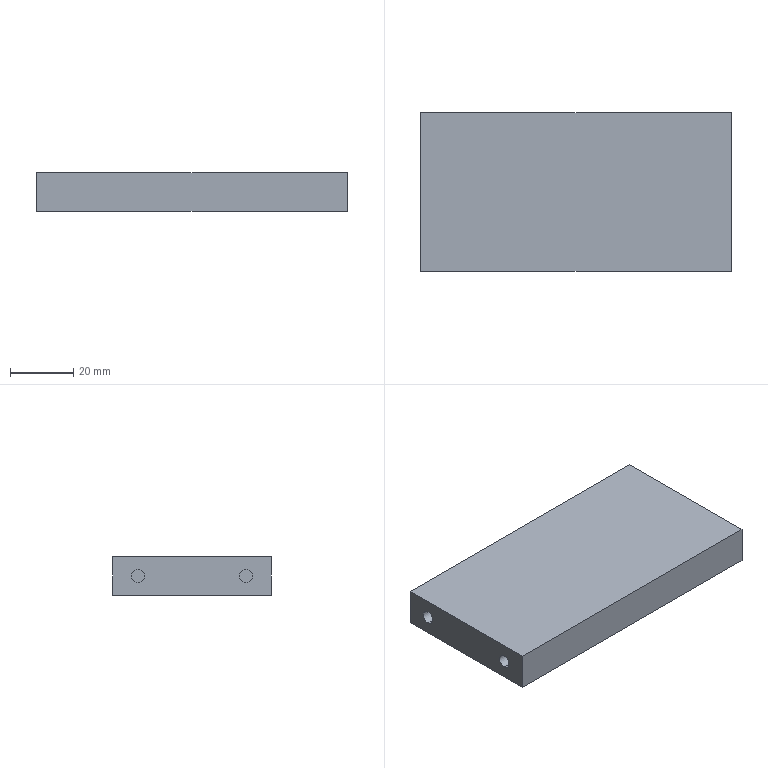Part | STEP file | Shim front mounting plate | 1 solid | 18 faces | box 98 x 50 x 12 mm | volume 58113 mm3 | plane 10 | cylinder 8 | commonest cylinder face diameters 4.2 x8
STEP:
#1=CARTESIAN_POINT('',(0.,0.,0.));
#2=DIRECTION('',(0.,0.,1.));
#3=DIRECTION('',(1.,0.,0.));
#4=AXIS2_PLACEMENT_3D('',#1,#2,#3);
#5=CARTESIAN_POINT('',(36.6,17.,3.9));
#6=VERTEX_POINT('',#5);
#7=CARTESIAN_POINT('',(49.,17.,3.9));
#8=VERTEX_POINT('',#7);
#9=CARTESIAN_POINT('',(49.,17.,3.9));
#10=DIRECTION('',(1.,0.,0.));
#11=VECTOR('',#10,1.);
#12=LINE('',#9,#11);
#13=CARTESIAN_POINT('',(49.,17.,6.));
#14=DIRECTION('',(1.,0.,0.));
#15=DIRECTION('',(0.,0.,-1.));
#16=AXIS2_PLACEMENT_3D('',#13,#14,#15);
#17=CYLINDRICAL_SURFACE('',#16,2.1);
#18=CARTESIAN_POINT('',(6.283,0.));
#19=DIRECTION('',(0.,1.));
#20=VECTOR('',#19,1.);
#21=LINE('',#18,#20);
#22=(GEOMETRIC_REPRESENTATION_CONTEXT(2)PARAMETRIC_REPRESENTATION_CONTEXT()REPRESENTATION_CONTEXT('',''));
#23=DEFINITIONAL_REPRESENTATION('',(#21),#22);
#24=PCURVE('',#17,#23);
#25=CARTESIAN_POINT('',(49.,17.,6.));
#26=DIRECTION('',(1.,0.,0.));
#27=DIRECTION('',(0.,0.,-1.));
#28=AXIS2_PLACEMENT_3D('',#25,#26,#27);
#29=CYLINDRICAL_SURFACE('',#28,2.1);
#30=CARTESIAN_POINT('',(0.,0.));
#31=DIRECTION('',(0.,1.));
#32=VECTOR('',#31,1.);
#33=LINE('',#30,#32);
#34=(GEOMETRIC_REPRESENTATION_CONTEXT(2)PARAMETRIC_REPRESENTATION_CONTEXT()REPRESENTATION_CONTEXT('',''));
#35=DEFINITIONAL_REPRESENTATION('',(#33),#34);
#36=PCURVE('',#29,#35);
#37=SURFACE_CURVE('',#12,(#24,#36),.PCURVE_S1.);
#38=EDGE_CURVE('',#6,#8,#37,.T.);
#39=ORIENTED_EDGE('',*,*,#38,.T.);
#40=CARTESIAN_POINT('',(49.,17.,8.1));
#41=VERTEX_POINT('',#40);
#42=CARTESIAN_POINT('',(49.,17.,6.));
#43=DIRECTION('',(1.,0.,0.));
#44=DIRECTION('',(0.,0.,-1.));
#45=AXIS2_PLACEMENT_3D('',#42,#43,#44);
#46=CIRCLE('',#45,2.1);
#47=CARTESIAN_POINT('',(0.,0.));
#48=DIRECTION('',(1.,0.));
#49=VECTOR('',#48,1.);
#50=LINE('',#47,#49);
#51=(GEOMETRIC_REPRESENTATION_CONTEXT(2)PARAMETRIC_REPRESENTATION_CONTEXT()REPRESENTATION_CONTEXT('',''));
#52=DEFINITIONAL_REPRESENTATION('',(#50),#51);
#53=PCURVE('',#17,#52);
#54=CARTESIAN_POINT('',(49.,-25.,12.));
#55=DIRECTION('',(-1.,0.,0.));
#56=DIRECTION('',(0.,0.,1.));
#57=AXIS2_PLACEMENT_3D('',#54,#55,#56);
#58=PLANE('',#57);
#59=CARTESIAN_POINT('',(-8.1,42.));
#60=CARTESIAN_POINT('',(-8.1,45.637));
#61=CARTESIAN_POINT('',(-4.95,43.819));
#62=CARTESIAN_POINT('',(-1.8,42.));
#63=CARTESIAN_POINT('',(-4.95,40.181));
#64=CARTESIAN_POINT('',(-8.1,38.363));
#65=CARTESIAN_POINT('',(-8.1,42.));
#66=(BOUNDED_CURVE()B_SPLINE_CURVE(2,(#59,#60,#61,#62,#63,#64,#65),.UNSPECIFIED.,.T.,.F.)B_SPLINE_CURVE_WITH_KNOTS((1,2,2,2,2,1),(-2.094,0.,2.094,4.189,6.283,8.378),.UNSPECIFIED.)CURVE()GEOMETRIC_REPRESENTATION_ITEM()RATIONAL_B_SPLINE_CURVE((1.,0.5,1.,0.5,1.,0.5,1.))REPRESENTATION_ITEM(''));
#67=(GEOMETRIC_REPRESENTATION_CONTEXT(2)PARAMETRIC_REPRESENTATION_CONTEXT()REPRESENTATION_CONTEXT('',''));
#68=DEFINITIONAL_REPRESENTATION('',(#66),#67);
#69=PCURVE('',#58,#68);
#70=SURFACE_CURVE('',#46,(#53,#69),.PCURVE_S1.);
#71=EDGE_CURVE('',#41,#8,#70,.T.);
#72=ORIENTED_EDGE('',*,*,#71,.F.);
#73=CARTESIAN_POINT('',(36.6,17.,8.1));
#74=VERTEX_POINT('',#73);
#75=CARTESIAN_POINT('',(49.,17.,8.1));
#76=DIRECTION('',(1.,0.,0.));
#77=VECTOR('',#76,1.);
#78=LINE('',#75,#77);
#79=CARTESIAN_POINT('',(3.142,0.));
#80=DIRECTION('',(0.,1.));
#81=VECTOR('',#80,1.);
#82=LINE('',#79,#81);
#83=(GEOMETRIC_REPRESENTATION_CONTEXT(2)PARAMETRIC_REPRESENTATION_CONTEXT()REPRESENTATION_CONTEXT('',''));
#84=DEFINITIONAL_REPRESENTATION('',(#82),#83);
#85=PCURVE('',#17,#84);
#86=CARTESIAN_POINT('',(3.142,0.));
#87=DIRECTION('',(0.,1.));
#88=VECTOR('',#87,1.);
#89=LINE('',#86,#88);
#90=(GEOMETRIC_REPRESENTATION_CONTEXT(2)PARAMETRIC_REPRESENTATION_CONTEXT()REPRESENTATION_CONTEXT('',''));
#91=DEFINITIONAL_REPRESENTATION('',(#89),#90);
#92=PCURVE('',#29,#91);
#93=SURFACE_CURVE('',#78,(#85,#92),.PCURVE_S1.);
#94=EDGE_CURVE('',#74,#41,#93,.T.);
#95=ORIENTED_EDGE('',*,*,#94,.F.);
#96=CARTESIAN_POINT('',(36.6,17.,6.));
#97=DIRECTION('',(1.,0.,0.));
#98=DIRECTION('',(0.,0.,-1.));
#99=AXIS2_PLACEMENT_3D('',#96,#97,#98);
#100=CIRCLE('',#99,2.1);
#101=CARTESIAN_POINT('',(0.,-12.4));
#102=DIRECTION('',(1.,0.));
#103=VECTOR('',#102,1.);
#104=LINE('',#101,#103);
#105=(GEOMETRIC_REPRESENTATION_CONTEXT(2)PARAMETRIC_REPRESENTATION_CONTEXT()REPRESENTATION_CONTEXT('',''));
#106=DEFINITIONAL_REPRESENTATION('',(#104),#105);
#107=PCURVE('',#17,#106);
#108=CARTESIAN_POINT('',(36.6,17.,6.));
#109=DIRECTION('',(-1.,0.,0.));
#110=DIRECTION('',(0.,0.,1.));
#111=AXIS2_PLACEMENT_3D('',#108,#109,#110);
#112=PLANE('',#111);
#113=CARTESIAN_POINT('',(-2.1,0.));
#114=CARTESIAN_POINT('',(-2.1,3.637));
#115=CARTESIAN_POINT('',(1.05,1.819));
#116=CARTESIAN_POINT('',(4.2,0.));
#117=CARTESIAN_POINT('',(1.05,-1.819));
#118=CARTESIAN_POINT('',(-2.1,-3.637));
#119=CARTESIAN_POINT('',(-2.1,0.));
#120=(BOUNDED_CURVE()B_SPLINE_CURVE(2,(#113,#114,#115,#116,#117,#118,#119),.UNSPECIFIED.,.T.,.F.)B_SPLINE_CURVE_WITH_KNOTS((1,2,2,2,2,1),(-2.094,0.,2.094,4.189,6.283,8.378),.UNSPECIFIED.)CURVE()GEOMETRIC_REPRESENTATION_ITEM()RATIONAL_B_SPLINE_CURVE((1.,0.5,1.,0.5,1.,0.5,1.))REPRESENTATION_ITEM(''));
#121=(GEOMETRIC_REPRESENTATION_CONTEXT(2)PARAMETRIC_REPRESENTATION_CONTEXT()REPRESENTATION_CONTEXT('',''));
#122=DEFINITIONAL_REPRESENTATION('',(#120),#121);
#123=PCURVE('',#112,#122);
#124=SURFACE_CURVE('',#100,(#107,#123),.PCURVE_S1.);
#125=EDGE_CURVE('',#74,#6,#124,.T.);
#126=ORIENTED_EDGE('',*,*,#125,.T.);
#127=EDGE_LOOP('',(#39,#72,#95,#126));
#128=FACE_BOUND('',#127,.F.);
#129=ADVANCED_FACE('',(#128),#17,.F.);
#130=CARTESIAN_POINT('',(36.6,-17.,3.9));
#131=VERTEX_POINT('',#130);
#132=CARTESIAN_POINT('',(49.,-17.,3.9));
#133=VERTEX_POINT('',#132);
#134=CARTESIAN_POINT('',(49.,-17.,3.9));
#135=DIRECTION('',(1.,0.,0.));
#136=VECTOR('',#135,1.);
#137=LINE('',#134,#136);
#138=CARTESIAN_POINT('',(49.,-17.,6.));
#139=DIRECTION('',(1.,0.,0.));
#140=DIRECTION('',(0.,0.,-1.));
#141=AXIS2_PLACEMENT_3D('',#138,#139,#140);
#142=CYLINDRICAL_SURFACE('',#141,2.1);
#143=CARTESIAN_POINT('',(6.283,0.));
#144=DIRECTION('',(0.,1.));
#145=VECTOR('',#144,1.);
#146=LINE('',#143,#145);
#147=(GEOMETRIC_REPRESENTATION_CONTEXT(2)PARAMETRIC_REPRESENTATION_CONTEXT()REPRESENTATION_CONTEXT('',''));
#148=DEFINITIONAL_REPRESENTATION('',(#146),#147);
#149=PCURVE('',#142,#148);
#150=CARTESIAN_POINT('',(49.,-17.,6.));
#151=DIRECTION('',(1.,0.,0.));
#152=DIRECTION('',(0.,0.,-1.));
#153=AXIS2_PLACEMENT_3D('',#150,#151,#152);
#154=CYLINDRICAL_SURFACE('',#153,2.1);
#155=CARTESIAN_POINT('',(0.,0.));
#156=DIRECTION('',(0.,1.));
#157=VECTOR('',#156,1.);
#158=LINE('',#155,#157);
#159=(GEOMETRIC_REPRESENTATION_CONTEXT(2)PARAMETRIC_REPRESENTATION_CONTEXT()REPRESENTATION_CONTEXT('',''));
#160=DEFINITIONAL_REPRESENTATION('',(#158),#159);
#161=PCURVE('',#154,#160);
#162=SURFACE_CURVE('',#137,(#149,#161),.PCURVE_S1.);
#163=EDGE_CURVE('',#131,#133,#162,.T.);
#164=ORIENTED_EDGE('',*,*,#163,.T.);
#165=CARTESIAN_POINT('',(49.,-17.,8.1));
#166=VERTEX_POINT('',#165);
#167=CARTESIAN_POINT('',(49.,-17.,6.));
#168=DIRECTION('',(1.,0.,0.));
#169=DIRECTION('',(0.,0.,-1.));
#170=AXIS2_PLACEMENT_3D('',#167,#168,#169);
#171=CIRCLE('',#170,2.1);
#172=CARTESIAN_POINT('',(0.,0.));
#173=DIRECTION('',(1.,0.));
#174=VECTOR('',#173,1.);
#175=LINE('',#172,#174);
#176=(GEOMETRIC_REPRESENTATION_CONTEXT(2)PARAMETRIC_REPRESENTATION_CONTEXT()REPRESENTATION_CONTEXT('',''));
#177=DEFINITIONAL_REPRESENTATION('',(#175),#176);
#178=PCURVE('',#142,#177);
#179=CARTESIAN_POINT('',(-8.1,8.));
#180=CARTESIAN_POINT('',(-8.1,11.637));
#181=CARTESIAN_POINT('',(-4.95,9.819));
#182=CARTESIAN_POINT('',(-1.8,8.));
#183=CARTESIAN_POINT('',(-4.95,6.181));
#184=CARTESIAN_POINT('',(-8.1,4.363));
#185=CARTESIAN_POINT('',(-8.1,8.));
#186=(BOUNDED_CURVE()B_SPLINE_CURVE(2,(#179,#180,#181,#182,#183,#184,#185),.UNSPECIFIED.,.T.,.F.)B_SPLINE_CURVE_WITH_KNOTS((1,2,2,2,2,1),(-2.094,0.,2.094,4.189,6.283,8.378),.UNSPECIFIED.)CURVE()GEOMETRIC_REPRESENTATION_ITEM()RATIONAL_B_SPLINE_CURVE((1.,0.5,1.,0.5,1.,0.5,1.))REPRESENTATION_ITEM(''));
#187=(GEOMETRIC_REPRESENTATION_CONTEXT(2)PARAMETRIC_REPRESENTATION_CONTEXT()REPRESENTATION_CONTEXT('',''));
#188=DEFINITIONAL_REPRESENTATION('',(#186),#187);
#189=PCURVE('',#58,#188);
#190=SURFACE_CURVE('',#171,(#178,#189),.PCURVE_S1.);
#191=EDGE_CURVE('',#166,#133,#190,.T.);
#192=ORIENTED_EDGE('',*,*,#191,.F.);
#193=CARTESIAN_POINT('',(36.6,-17.,8.1));
#194=VERTEX_POINT('',#193);
#195=CARTESIAN_POINT('',(49.,-17.,8.1));
#196=DIRECTION('',(1.,0.,0.));
#197=VECTOR('',#196,1.);
#198=LINE('',#195,#197);
#199=CARTESIAN_POINT('',(3.142,0.));
#200=DIRECTION('',(0.,1.));
#201=VECTOR('',#200,1.);
#202=LINE('',#199,#201);
#203=(GEOMETRIC_REPRESENTATION_CONTEXT(2)PARAMETRIC_REPRESENTATION_CONTEXT()REPRESENTATION_CONTEXT('',''));
#204=DEFINITIONAL_REPRESENTATION('',(#202),#203);
#205=PCURVE('',#142,#204);
#206=CARTESIAN_POINT('',(3.142,0.));
#207=DIRECTION('',(0.,1.));
#208=VECTOR('',#207,1.);
#209=LINE('',#206,#208);
#210=(GEOMETRIC_REPRESENTATION_CONTEXT(2)PARAMETRIC_REPRESENTATION_CONTEXT()REPRESENTATION_CONTEXT('',''));
#211=DEFINITIONAL_REPRESENTATION('',(#209),#210);
#212=PCURVE('',#154,#211);
#213=SURFACE_CURVE('',#198,(#205,#212),.PCURVE_S1.);
#214=EDGE_CURVE('',#194,#166,#213,.T.);
#215=ORIENTED_EDGE('',*,*,#214,.F.);
#216=CARTESIAN_POINT('',(36.6,-17.,6.));
#217=DIRECTION('',(1.,0.,0.));
#218=DIRECTION('',(0.,0.,-1.));
#219=AXIS2_PLACEMENT_3D('',#216,#217,#218);
#220=CIRCLE('',#219,2.1);
#221=CARTESIAN_POINT('',(0.,-12.4));
#222=DIRECTION('',(1.,0.));
#223=VECTOR('',#222,1.);
#224=LINE('',#221,#223);
#225=(GEOMETRIC_REPRESENTATION_CONTEXT(2)PARAMETRIC_REPRESENTATION_CONTEXT()REPRESENTATION_CONTEXT('',''));
#226=DEFINITIONAL_REPRESENTATION('',(#224),#225);
#227=PCURVE('',#142,#226);
#228=CARTESIAN_POINT('',(36.6,-17.,6.));
#229=DIRECTION('',(-1.,0.,0.));
#230=DIRECTION('',(0.,0.,1.));
#231=AXIS2_PLACEMENT_3D('',#228,#229,#230);
#232=PLANE('',#231);
#233=CARTESIAN_POINT('',(-2.1,0.));
#234=CARTESIAN_POINT('',(-2.1,3.637));
#235=CARTESIAN_POINT('',(1.05,1.819));
#236=CARTESIAN_POINT('',(4.2,0.));
#237=CARTESIAN_POINT('',(1.05,-1.819));
#238=CARTESIAN_POINT('',(-2.1,-3.637));
#239=CARTESIAN_POINT('',(-2.1,0.));
#240=(BOUNDED_CURVE()B_SPLINE_CURVE(2,(#233,#234,#235,#236,#237,#238,#239),.UNSPECIFIED.,.T.,.F.)B_SPLINE_CURVE_WITH_KNOTS((1,2,2,2,2,1),(-2.094,0.,2.094,4.189,6.283,8.378),.UNSPECIFIED.)CURVE()GEOMETRIC_REPRESENTATION_ITEM()RATIONAL_B_SPLINE_CURVE((1.,0.5,1.,0.5,1.,0.5,1.))REPRESENTATION_ITEM(''));
#241=(GEOMETRIC_REPRESENTATION_CONTEXT(2)PARAMETRIC_REPRESENTATION_CONTEXT()REPRESENTATION_CONTEXT('',''));
#242=DEFINITIONAL_REPRESENTATION('',(#240),#241);
#243=PCURVE('',#232,#242);
#244=SURFACE_CURVE('',#220,(#227,#243),.PCURVE_S1.);
#245=EDGE_CURVE('',#194,#131,#244,.T.);
#246=ORIENTED_EDGE('',*,*,#245,.T.);
#247=EDGE_LOOP('',(#164,#192,#215,#246));
#248=FACE_BOUND('',#247,.F.);
#249=ADVANCED_FACE('',(#248),#142,.F.);
#250=CARTESIAN_POINT('',(-36.6,17.,8.1));
#251=VERTEX_POINT('',#250);
#252=CARTESIAN_POINT('',(-49.,17.,8.1));
#253=VERTEX_POINT('',#252);
#254=CARTESIAN_POINT('',(-49.,17.,8.1));
#255=DIRECTION('',(-1.,0.,0.));
#256=VECTOR('',#255,1.);
#257=LINE('',#254,#256);
#258=CARTESIAN_POINT('',(-49.,17.,6.));
#259=DIRECTION('',(-1.,0.,0.));
#260=DIRECTION('',(0.,0.,1.));
#261=AXIS2_PLACEMENT_3D('',#258,#259,#260);
#262=CYLINDRICAL_SURFACE('',#261,2.1);
#263=CARTESIAN_POINT('',(6.283,0.));
#264=DIRECTION('',(0.,1.));
#265=VECTOR('',#264,1.);
#266=LINE('',#263,#265);
#267=(GEOMETRIC_REPRESENTATION_CONTEXT(2)PARAMETRIC_REPRESENTATION_CONTEXT()REPRESENTATION_CONTEXT('',''));
#268=DEFINITIONAL_REPRESENTATION('',(#266),#267);
#269=PCURVE('',#262,#268);
#270=CARTESIAN_POINT('',(-49.,17.,6.));
#271=DIRECTION('',(-1.,0.,0.));
#272=DIRECTION('',(0.,0.,1.));
#273=AXIS2_PLACEMENT_3D('',#270,#271,#272);
#274=CYLINDRICAL_SURFACE('',#273,2.1);
#275=CARTESIAN_POINT('',(0.,0.));
#276=DIRECTION('',(0.,1.));
#277=VECTOR('',#276,1.);
#278=LINE('',#275,#277);
#279=(GEOMETRIC_REPRESENTATION_CONTEXT(2)PARAMETRIC_REPRESENTATION_CONTEXT()REPRESENTATION_CONTEXT('',''));
#280=DEFINITIONAL_REPRESENTATION('',(#278),#279);
#281=PCURVE('',#274,#280);
#282=SURFACE_CURVE('',#257,(#269,#281),.PCURVE_S1.);
#283=EDGE_CURVE('',#251,#253,#282,.T.);
#284=ORIENTED_EDGE('',*,*,#283,.T.);
#285=CARTESIAN_POINT('',(-49.,17.,3.9));
#286=VERTEX_POINT('',#285);
#287=CARTESIAN_POINT('',(-49.,17.,6.));
#288=DIRECTION('',(-1.,0.,0.));
#289=DIRECTION('',(0.,0.,1.));
#290=AXIS2_PLACEMENT_3D('',#287,#288,#289);
#291=CIRCLE('',#290,2.1);
#292=CARTESIAN_POINT('',(0.,0.));
#293=DIRECTION('',(1.,0.));
#294=VECTOR('',#293,1.);
#295=LINE('',#292,#294);
#296=(GEOMETRIC_REPRESENTATION_CONTEXT(2)PARAMETRIC_REPRESENTATION_CONTEXT()REPRESENTATION_CONTEXT('',''));
#297=DEFINITIONAL_REPRESENTATION('',(#295),#296);
#298=PCURVE('',#262,#297);
#299=CARTESIAN_POINT('',(-49.,-25.,12.));
#300=DIRECTION('',(1.,0.,0.));
#301=DIRECTION('',(0.,0.,-1.));
#302=AXIS2_PLACEMENT_3D('',#299,#300,#301);
#303=PLANE('',#302);
#304=CARTESIAN_POINT('',(3.9,42.));
#305=CARTESIAN_POINT('',(3.9,45.637));
#306=CARTESIAN_POINT('',(7.05,43.819));
#307=CARTESIAN_POINT('',(10.2,42.));
#308=CARTESIAN_POINT('',(7.05,40.181));
#309=CARTESIAN_POINT('',(3.9,38.363));
#310=CARTESIAN_POINT('',(3.9,42.));
#311=(BOUNDED_CURVE()B_SPLINE_CURVE(2,(#304,#305,#306,#307,#308,#309,#310),.UNSPECIFIED.,.T.,.F.)B_SPLINE_CURVE_WITH_KNOTS((1,2,2,2,2,1),(-2.094,0.,2.094,4.189,6.283,8.378),.UNSPECIFIED.)CURVE()GEOMETRIC_REPRESENTATION_ITEM()RATIONAL_B_SPLINE_CURVE((1.,0.5,1.,0.5,1.,0.5,1.))REPRESENTATION_ITEM(''));
#312=(GEOMETRIC_REPRESENTATION_CONTEXT(2)PARAMETRIC_REPRESENTATION_CONTEXT()REPRESENTATION_CONTEXT('',''));
#313=DEFINITIONAL_REPRESENTATION('',(#311),#312);
#314=PCURVE('',#303,#313);
#315=SURFACE_CURVE('',#291,(#298,#314),.PCURVE_S1.);
#316=EDGE_CURVE('',#286,#253,#315,.T.);
#317=ORIENTED_EDGE('',*,*,#316,.F.);
#318=CARTESIAN_POINT('',(-36.6,17.,3.9));
#319=VERTEX_POINT('',#318);
#320=CARTESIAN_POINT('',(-49.,17.,3.9));
#321=DIRECTION('',(-1.,0.,0.));
#322=VECTOR('',#321,1.);
#323=LINE('',#320,#322);
#324=CARTESIAN_POINT('',(3.142,0.));
#325=DIRECTION('',(0.,1.));
#326=VECTOR('',#325,1.);
#327=LINE('',#324,#326);
#328=(GEOMETRIC_REPRESENTATION_CONTEXT(2)PARAMETRIC_REPRESENTATION_CONTEXT()REPRESENTATION_CONTEXT('',''));
#329=DEFINITIONAL_REPRESENTATION('',(#327),#328);
#330=PCURVE('',#262,#329);
#331=CARTESIAN_POINT('',(3.142,0.));
#332=DIRECTION('',(0.,1.));
#333=VECTOR('',#332,1.);
#334=LINE('',#331,#333);
#335=(GEOMETRIC_REPRESENTATION_CONTEXT(2)PARAMETRIC_REPRESENTATION_CONTEXT()REPRESENTATION_CONTEXT('',''));
#336=DEFINITIONAL_REPRESENTATION('',(#334),#335);
#337=PCURVE('',#274,#336);
#338=SURFACE_CURVE('',#323,(#330,#337),.PCURVE_S1.);
#339=EDGE_CURVE('',#319,#286,#338,.T.);
#340=ORIENTED_EDGE('',*,*,#339,.F.);
#341=CARTESIAN_POINT('',(-36.6,17.,6.));
#342=DIRECTION('',(-1.,0.,0.));
#343=DIRECTION('',(0.,0.,1.));
#344=AXIS2_PLACEMENT_3D('',#341,#342,#343);
#345=CIRCLE('',#344,2.1);
#346=CARTESIAN_POINT('',(0.,-12.4));
#347=DIRECTION('',(1.,0.));
#348=VECTOR('',#347,1.);
#349=LINE('',#346,#348);
#350=(GEOMETRIC_REPRESENTATION_CONTEXT(2)PARAMETRIC_REPRESENTATION_CONTEXT()REPRESENTATION_CONTEXT('',''));
#351=DEFINITIONAL_REPRESENTATION('',(#349),#350);
#352=PCURVE('',#262,#351);
#353=CARTESIAN_POINT('',(-36.6,17.,6.));
#354=DIRECTION('',(1.,0.,0.));
#355=DIRECTION('',(0.,0.,-1.));
#356=AXIS2_PLACEMENT_3D('',#353,#354,#355);
#357=PLANE('',#356);
#358=CARTESIAN_POINT('',(-2.1,0.));
#359=CARTESIAN_POINT('',(-2.1,3.637));
#360=CARTESIAN_POINT('',(1.05,1.819));
#361=CARTESIAN_POINT('',(4.2,0.));
#362=CARTESIAN_POINT('',(1.05,-1.819));
#363=CARTESIAN_POINT('',(-2.1,-3.637));
#364=CARTESIAN_POINT('',(-2.1,0.));
#365=(BOUNDED_CURVE()B_SPLINE_CURVE(2,(#358,#359,#360,#361,#362,#363,#364),.UNSPECIFIED.,.T.,.F.)B_SPLINE_CURVE_WITH_KNOTS((1,2,2,2,2,1),(-2.094,0.,2.094,4.189,6.283,8.378),.UNSPECIFIED.)CURVE()GEOMETRIC_REPRESENTATION_ITEM()RATIONAL_B_SPLINE_CURVE((1.,0.5,1.,0.5,1.,0.5,1.))REPRESENTATION_ITEM(''));
#366=(GEOMETRIC_REPRESENTATION_CONTEXT(2)PARAMETRIC_REPRESENTATION_CONTEXT()REPRESENTATION_CONTEXT('',''));
#367=DEFINITIONAL_REPRESENTATION('',(#365),#366);
#368=PCURVE('',#357,#367);
#369=SURFACE_CURVE('',#345,(#352,#368),.PCURVE_S1.);
#370=EDGE_CURVE('',#319,#251,#369,.T.);
#371=ORIENTED_EDGE('',*,*,#370,.T.);
#372=EDGE_LOOP('',(#284,#317,#340,#371));
#373=FACE_BOUND('',#372,.F.);
#374=ADVANCED_FACE('',(#373),#262,.F.);
#375=CARTESIAN_POINT('',(-36.6,-17.,8.1));
#376=VERTEX_POINT('',#375);
#377=CARTESIAN_POINT('',(-49.,-17.,8.1));
#378=VERTEX_POINT('',#377);
#379=CARTESIAN_POINT('',(-49.,-17.,8.1));
#380=DIRECTION('',(-1.,0.,0.));
#381=VECTOR('',#380,1.);
#382=LINE('',#379,#381);
#383=CARTESIAN_POINT('',(-49.,-17.,6.));
#384=DIRECTION('',(-1.,0.,0.));
#385=DIRECTION('',(0.,0.,1.));
#386=AXIS2_PLACEMENT_3D('',#383,#384,#385);
#387=CYLINDRICAL_SURFACE('',#386,2.1);
#388=CARTESIAN_POINT('',(6.283,0.));
#389=DIRECTION('',(0.,1.));
#390=VECTOR('',#389,1.);
#391=LINE('',#388,#390);
#392=(GEOMETRIC_REPRESENTATION_CONTEXT(2)PARAMETRIC_REPRESENTATION_CONTEXT()REPRESENTATION_CONTEXT('',''));
#393=DEFINITIONAL_REPRESENTATION('',(#391),#392);
#394=PCURVE('',#387,#393);
#395=CARTESIAN_POINT('',(-49.,-17.,6.));
#396=DIRECTION('',(-1.,0.,0.));
#397=DIRECTION('',(0.,0.,1.));
#398=AXIS2_PLACEMENT_3D('',#395,#396,#397);
#399=CYLINDRICAL_SURFACE('',#398,2.1);
#400=CARTESIAN_POINT('',(0.,0.));
#401=DIRECTION('',(0.,1.));
#402=VECTOR('',#401,1.);
#403=LINE('',#400,#402);
#404=(GEOMETRIC_REPRESENTATION_CONTEXT(2)PARAMETRIC_REPRESENTATION_CONTEXT()REPRESENTATION_CONTEXT('',''));
#405=DEFINITIONAL_REPRESENTATION('',(#403),#404);
#406=PCURVE('',#399,#405);
#407=SURFACE_CURVE('',#382,(#394,#406),.PCURVE_S1.);
#408=EDGE_CURVE('',#376,#378,#407,.T.);
#409=ORIENTED_EDGE('',*,*,#408,.T.);
#410=CARTESIAN_POINT('',(-49.,-17.,3.9));
#411=VERTEX_POINT('',#410);
#412=CARTESIAN_POINT('',(-49.,-17.,6.));
#413=DIRECTION('',(-1.,0.,0.));
#414=DIRECTION('',(0.,0.,1.));
#415=AXIS2_PLACEMENT_3D('',#412,#413,#414);
#416=CIRCLE('',#415,2.1);
#417=CARTESIAN_POINT('',(0.,0.));
#418=DIRECTION('',(1.,0.));
#419=VECTOR('',#418,1.);
#420=LINE('',#417,#419);
#421=(GEOMETRIC_REPRESENTATION_CONTEXT(2)PARAMETRIC_REPRESENTATION_CONTEXT()REPRESENTATION_CONTEXT('',''));
#422=DEFINITIONAL_REPRESENTATION('',(#420),#421);
#423=PCURVE('',#387,#422);
#424=CARTESIAN_POINT('',(3.9,8.));
#425=CARTESIAN_POINT('',(3.9,11.637));
#426=CARTESIAN_POINT('',(7.05,9.819));
#427=CARTESIAN_POINT('',(10.2,8.));
#428=CARTESIAN_POINT('',(7.05,6.181));
#429=CARTESIAN_POINT('',(3.9,4.363));
#430=CARTESIAN_POINT('',(3.9,8.));
#431=(BOUNDED_CURVE()B_SPLINE_CURVE(2,(#424,#425,#426,#427,#428,#429,#430),.UNSPECIFIED.,.T.,.F.)B_SPLINE_CURVE_WITH_KNOTS((1,2,2,2,2,1),(-2.094,0.,2.094,4.189,6.283,8.378),.UNSPECIFIED.)CURVE()GEOMETRIC_REPRESENTATION_ITEM()RATIONAL_B_SPLINE_CURVE((1.,0.5,1.,0.5,1.,0.5,1.))REPRESENTATION_ITEM(''));
#432=(GEOMETRIC_REPRESENTATION_CONTEXT(2)PARAMETRIC_REPRESENTATION_CONTEXT()REPRESENTATION_CONTEXT('',''));
#433=DEFINITIONAL_REPRESENTATION('',(#431),#432);
#434=PCURVE('',#303,#433);
#435=SURFACE_CURVE('',#416,(#423,#434),.PCURVE_S1.);
#436=EDGE_CURVE('',#411,#378,#435,.T.);
#437=ORIENTED_EDGE('',*,*,#436,.F.);
#438=CARTESIAN_POINT('',(-36.6,-17.,3.9));
#439=VERTEX_POINT('',#438);
#440=CARTESIAN_POINT('',(-49.,-17.,3.9));
#441=DIRECTION('',(-1.,0.,0.));
#442=VECTOR('',#441,1.);
#443=LINE('',#440,#442);
#444=CARTESIAN_POINT('',(3.142,0.));
#445=DIRECTION('',(0.,1.));
#446=VECTOR('',#445,1.);
#447=LINE('',#444,#446);
#448=(GEOMETRIC_REPRESENTATION_CONTEXT(2)PARAMETRIC_REPRESENTATION_CONTEXT()REPRESENTATION_CONTEXT('',''));
#449=DEFINITIONAL_REPRESENTATION('',(#447),#448);
#450=PCURVE('',#387,#449);
#451=CARTESIAN_POINT('',(3.142,0.));
#452=DIRECTION('',(0.,1.));
#453=VECTOR('',#452,1.);
#454=LINE('',#451,#453);
#455=(GEOMETRIC_REPRESENTATION_CONTEXT(2)PARAMETRIC_REPRESENTATION_CONTEXT()REPRESENTATION_CONTEXT('',''));
#456=DEFINITIONAL_REPRESENTATION('',(#454),#455);
#457=PCURVE('',#399,#456);
#458=SURFACE_CURVE('',#443,(#450,#457),.PCURVE_S1.);
#459=EDGE_CURVE('',#439,#411,#458,.T.);
#460=ORIENTED_EDGE('',*,*,#459,.F.);
#461=CARTESIAN_POINT('',(-36.6,-17.,6.));
#462=DIRECTION('',(-1.,0.,0.));
#463=DIRECTION('',(0.,0.,1.));
#464=AXIS2_PLACEMENT_3D('',#461,#462,#463);
#465=CIRCLE('',#464,2.1);
#466=CARTESIAN_POINT('',(0.,-12.4));
#467=DIRECTION('',(1.,0.));
#468=VECTOR('',#467,1.);
#469=LINE('',#466,#468);
#470=(GEOMETRIC_REPRESENTATION_CONTEXT(2)PARAMETRIC_REPRESENTATION_CONTEXT()REPRESENTATION_CONTEXT('',''));
#471=DEFINITIONAL_REPRESENTATION('',(#469),#470);
#472=PCURVE('',#387,#471);
#473=CARTESIAN_POINT('',(-36.6,-17.,6.));
#474=DIRECTION('',(1.,0.,0.));
#475=DIRECTION('',(0.,0.,-1.));
#476=AXIS2_PLACEMENT_3D('',#473,#474,#475);
#477=PLANE('',#476);
#478=CARTESIAN_POINT('',(-2.1,0.));
#479=CARTESIAN_POINT('',(-2.1,3.637));
#480=CARTESIAN_POINT('',(1.05,1.819));
#481=CARTESIAN_POINT('',(4.2,0.));
#482=CARTESIAN_POINT('',(1.05,-1.819));
#483=CARTESIAN_POINT('',(-2.1,-3.637));
#484=CARTESIAN_POINT('',(-2.1,0.));
#485=(BOUNDED_CURVE()B_SPLINE_CURVE(2,(#478,#479,#480,#481,#482,#483,#484),.UNSPECIFIED.,.T.,.F.)B_SPLINE_CURVE_WITH_KNOTS((1,2,2,2,2,1),(-2.094,0.,2.094,4.189,6.283,8.378),.UNSPECIFIED.)CURVE()GEOMETRIC_REPRESENTATION_ITEM()RATIONAL_B_SPLINE_CURVE((1.,0.5,1.,0.5,1.,0.5,1.))REPRESENTATION_ITEM(''));
#486=(GEOMETRIC_REPRESENTATION_CONTEXT(2)PARAMETRIC_REPRESENTATION_CONTEXT()REPRESENTATION_CONTEXT('',''));
#487=DEFINITIONAL_REPRESENTATION('',(#485),#486);
#488=PCURVE('',#477,#487);
#489=SURFACE_CURVE('',#465,(#472,#488),.PCURVE_S1.);
#490=EDGE_CURVE('',#439,#376,#489,.T.);
#491=ORIENTED_EDGE('',*,*,#490,.T.);
#492=EDGE_LOOP('',(#409,#437,#460,#491));
#493=FACE_BOUND('',#492,.F.);
#494=ADVANCED_FACE('',(#493),#387,.F.);
#495=CARTESIAN_POINT('',(-49.,25.,12.));
#496=VERTEX_POINT('',#495);
#497=CARTESIAN_POINT('',(49.,25.,12.));
#498=VERTEX_POINT('',#497);
#499=CARTESIAN_POINT('',(49.,25.,12.));
#500=DIRECTION('',(1.,0.,0.));
#501=VECTOR('',#500,1.);
#502=LINE('',#499,#501);
#503=CARTESIAN_POINT('',(49.,25.,12.));
#504=DIRECTION('',(0.,0.,-1.));
#505=DIRECTION('',(-1.,0.,0.));
#506=AXIS2_PLACEMENT_3D('',#503,#504,#505);
#507=PLANE('',#506);
#508=CARTESIAN_POINT('',(0.,0.));
#509=DIRECTION('',(-1.,0.));
#510=VECTOR('',#509,1.);
#511=LINE('',#508,#510);
#512=(GEOMETRIC_REPRESENTATION_CONTEXT(2)PARAMETRIC_REPRESENTATION_CONTEXT()REPRESENTATION_CONTEXT('',''));
#513=DEFINITIONAL_REPRESENTATION('',(#511),#512);
#514=PCURVE('',#507,#513);
#515=CARTESIAN_POINT('',(-49.,25.,12.));
#516=DIRECTION('',(0.,-1.,0.));
#517=DIRECTION('',(0.,0.,-1.));
#518=AXIS2_PLACEMENT_3D('',#515,#516,#517);
#519=PLANE('',#518);
#520=CARTESIAN_POINT('',(0.,98.));
#521=DIRECTION('',(0.,1.));
#522=VECTOR('',#521,1.);
#523=LINE('',#520,#522);
#524=(GEOMETRIC_REPRESENTATION_CONTEXT(2)PARAMETRIC_REPRESENTATION_CONTEXT()REPRESENTATION_CONTEXT('',''));
#525=DEFINITIONAL_REPRESENTATION('',(#523),#524);
#526=PCURVE('',#519,#525);
#527=SURFACE_CURVE('',#502,(#514,#526),.PCURVE_S1.);
#528=EDGE_CURVE('',#496,#498,#527,.T.);
#529=ORIENTED_EDGE('',*,*,#528,.F.);
#530=CARTESIAN_POINT('',(-49.,-25.,12.));
#531=VERTEX_POINT('',#530);
#532=CARTESIAN_POINT('',(-49.,25.,12.));
#533=DIRECTION('',(0.,1.,0.));
#534=VECTOR('',#533,1.);
#535=LINE('',#532,#534);
#536=CARTESIAN_POINT('',(98.,0.));
#537=DIRECTION('',(0.,1.));
#538=VECTOR('',#537,1.);
#539=LINE('',#536,#538);
#540=(GEOMETRIC_REPRESENTATION_CONTEXT(2)PARAMETRIC_REPRESENTATION_CONTEXT()REPRESENTATION_CONTEXT('',''));
#541=DEFINITIONAL_REPRESENTATION('',(#539),#540);
#542=PCURVE('',#507,#541);
#543=CARTESIAN_POINT('',(0.,50.));
#544=DIRECTION('',(0.,1.));
#545=VECTOR('',#544,1.);
#546=LINE('',#543,#545);
#547=(GEOMETRIC_REPRESENTATION_CONTEXT(2)PARAMETRIC_REPRESENTATION_CONTEXT()REPRESENTATION_CONTEXT('',''));
#548=DEFINITIONAL_REPRESENTATION('',(#546),#547);
#549=PCURVE('',#303,#548);
#550=SURFACE_CURVE('',#535,(#542,#549),.PCURVE_S1.);
#551=EDGE_CURVE('',#531,#496,#550,.T.);
#552=ORIENTED_EDGE('',*,*,#551,.F.);
#553=CARTESIAN_POINT('',(49.,-25.,12.));
#554=VERTEX_POINT('',#553);
#555=CARTESIAN_POINT('',(49.,-25.,12.));
#556=DIRECTION('',(-1.,0.,0.));
#557=VECTOR('',#556,1.);
#558=LINE('',#555,#557);
#559=CARTESIAN_POINT('',(0.,-50.));
#560=DIRECTION('',(1.,0.));
#561=VECTOR('',#560,1.);
#562=LINE('',#559,#561);
#563=(GEOMETRIC_REPRESENTATION_CONTEXT(2)PARAMETRIC_REPRESENTATION_CONTEXT()REPRESENTATION_CONTEXT('',''));
#564=DEFINITIONAL_REPRESENTATION('',(#562),#563);
#565=PCURVE('',#507,#564);
#566=CARTESIAN_POINT('',(-49.,-25.,12.));
#567=DIRECTION('',(0.,1.,0.));
#568=DIRECTION('',(0.,0.,1.));
#569=AXIS2_PLACEMENT_3D('',#566,#567,#568);
#570=PLANE('',#569);
#571=CARTESIAN_POINT('',(0.,98.));
#572=DIRECTION('',(0.,-1.));
#573=VECTOR('',#572,1.);
#574=LINE('',#571,#573);
#575=(GEOMETRIC_REPRESENTATION_CONTEXT(2)PARAMETRIC_REPRESENTATION_CONTEXT()REPRESENTATION_CONTEXT('',''));
#576=DEFINITIONAL_REPRESENTATION('',(#574),#575);
#577=PCURVE('',#570,#576);
#578=SURFACE_CURVE('',#558,(#565,#577),.PCURVE_S1.);
#579=EDGE_CURVE('',#554,#531,#578,.T.);
#580=ORIENTED_EDGE('',*,*,#579,.F.);
#581=CARTESIAN_POINT('',(49.,25.,12.));
#582=DIRECTION('',(0.,-1.,0.));
#583=VECTOR('',#582,1.);
#584=LINE('',#581,#583);
#585=CARTESIAN_POINT('',(0.,0.));
#586=DIRECTION('',(0.,-1.));
#587=VECTOR('',#586,1.);
#588=LINE('',#585,#587);
#589=(GEOMETRIC_REPRESENTATION_CONTEXT(2)PARAMETRIC_REPRESENTATION_CONTEXT()REPRESENTATION_CONTEXT('',''));
#590=DEFINITIONAL_REPRESENTATION('',(#588),#589);
#591=PCURVE('',#507,#590);
#592=CARTESIAN_POINT('',(0.,50.));
#593=DIRECTION('',(0.,-1.));
#594=VECTOR('',#593,1.);
#595=LINE('',#592,#594);
#596=(GEOMETRIC_REPRESENTATION_CONTEXT(2)PARAMETRIC_REPRESENTATION_CONTEXT()REPRESENTATION_CONTEXT('',''));
#597=DEFINITIONAL_REPRESENTATION('',(#595),#596);
#598=PCURVE('',#58,#597);
#599=SURFACE_CURVE('',#584,(#591,#598),.PCURVE_S1.);
#600=EDGE_CURVE('',#498,#554,#599,.T.);
#601=ORIENTED_EDGE('',*,*,#600,.F.);
#602=EDGE_LOOP('',(#529,#552,#580,#601));
#603=FACE_BOUND('',#602,.T.);
#604=ADVANCED_FACE('',(#603),#507,.F.);
#605=CARTESIAN_POINT('',(49.,25.,0.));
#606=VERTEX_POINT('',#605);
#607=CARTESIAN_POINT('',(49.,25.,12.));
#608=DIRECTION('',(0.,0.,-1.));
#609=VECTOR('',#608,1.);
#610=LINE('',#607,#609);
#611=CARTESIAN_POINT('',(0.,50.));
#612=DIRECTION('',(-1.,0.));
#613=VECTOR('',#612,1.);
#614=LINE('',#611,#613);
#615=(GEOMETRIC_REPRESENTATION_CONTEXT(2)PARAMETRIC_REPRESENTATION_CONTEXT()REPRESENTATION_CONTEXT('',''));
#616=DEFINITIONAL_REPRESENTATION('',(#614),#615);
#617=PCURVE('',#58,#616);
#618=CARTESIAN_POINT('',(0.,98.));
#619=DIRECTION('',(1.,0.));
#620=VECTOR('',#619,1.);
#621=LINE('',#618,#620);
#622=(GEOMETRIC_REPRESENTATION_CONTEXT(2)PARAMETRIC_REPRESENTATION_CONTEXT()REPRESENTATION_CONTEXT('',''));
#623=DEFINITIONAL_REPRESENTATION('',(#621),#622);
#624=PCURVE('',#519,#623);
#625=SURFACE_CURVE('',#610,(#617,#624),.PCURVE_S1.);
#626=EDGE_CURVE('',#498,#606,#625,.T.);
#627=ORIENTED_EDGE('',*,*,#626,.F.);
#628=ORIENTED_EDGE('',*,*,#600,.T.);
#629=CARTESIAN_POINT('',(49.,-25.,0.));
#630=VERTEX_POINT('',#629);
#631=CARTESIAN_POINT('',(49.,-25.,12.));
#632=DIRECTION('',(0.,0.,1.));
#633=VECTOR('',#632,1.);
#634=LINE('',#631,#633);
#635=CARTESIAN_POINT('',(0.,0.));
#636=DIRECTION('',(1.,0.));
#637=VECTOR('',#636,1.);
#638=LINE('',#635,#637);
#639=(GEOMETRIC_REPRESENTATION_CONTEXT(2)PARAMETRIC_REPRESENTATION_CONTEXT()REPRESENTATION_CONTEXT('',''));
#640=DEFINITIONAL_REPRESENTATION('',(#638),#639);
#641=PCURVE('',#58,#640);
#642=CARTESIAN_POINT('',(0.,98.));
#643=DIRECTION('',(1.,0.));
#644=VECTOR('',#643,1.);
#645=LINE('',#642,#644);
#646=(GEOMETRIC_REPRESENTATION_CONTEXT(2)PARAMETRIC_REPRESENTATION_CONTEXT()REPRESENTATION_CONTEXT('',''));
#647=DEFINITIONAL_REPRESENTATION('',(#645),#646);
#648=PCURVE('',#570,#647);
#649=SURFACE_CURVE('',#634,(#641,#648),.PCURVE_S1.);
#650=EDGE_CURVE('',#630,#554,#649,.T.);
#651=ORIENTED_EDGE('',*,*,#650,.F.);
#652=CARTESIAN_POINT('',(49.,-25.,0.));
#653=DIRECTION('',(0.,-1.,0.));
#654=VECTOR('',#653,1.);
#655=LINE('',#652,#654);
#656=CARTESIAN_POINT('',(-12.,0.));
#657=DIRECTION('',(0.,-1.));
#658=VECTOR('',#657,1.);
#659=LINE('',#656,#658);
#660=(GEOMETRIC_REPRESENTATION_CONTEXT(2)PARAMETRIC_REPRESENTATION_CONTEXT()REPRESENTATION_CONTEXT('',''));
#661=DEFINITIONAL_REPRESENTATION('',(#659),#660);
#662=PCURVE('',#58,#661);
#663=CARTESIAN_POINT('',(49.,25.,0.));
#664=DIRECTION('',(0.,0.,-1.));
#665=DIRECTION('',(-1.,0.,0.));
#666=AXIS2_PLACEMENT_3D('',#663,#664,#665);
#667=PLANE('',#666);
#668=CARTESIAN_POINT('',(0.,-50.));
#669=DIRECTION('',(0.,-1.));
#670=VECTOR('',#669,1.);
#671=LINE('',#668,#670);
#672=(GEOMETRIC_REPRESENTATION_CONTEXT(2)PARAMETRIC_REPRESENTATION_CONTEXT()REPRESENTATION_CONTEXT('',''));
#673=DEFINITIONAL_REPRESENTATION('',(#671),#672);
#674=PCURVE('',#667,#673);
#675=SURFACE_CURVE('',#655,(#662,#674),.PCURVE_S1.);
#676=EDGE_CURVE('',#606,#630,#675,.T.);
#677=ORIENTED_EDGE('',*,*,#676,.F.);
#678=EDGE_LOOP('',(#627,#628,#651,#677));
#679=FACE_BOUND('',#678,.T.);
#680=CARTESIAN_POINT('',(49.,17.,6.));
#681=DIRECTION('',(1.,0.,0.));
#682=DIRECTION('',(0.,0.,-1.));
#683=AXIS2_PLACEMENT_3D('',#680,#681,#682);
#684=CIRCLE('',#683,2.1);
#685=CARTESIAN_POINT('',(-8.1,42.));
#686=CARTESIAN_POINT('',(-8.1,45.637));
#687=CARTESIAN_POINT('',(-4.95,43.819));
#688=CARTESIAN_POINT('',(-1.8,42.));
#689=CARTESIAN_POINT('',(-4.95,40.181));
#690=CARTESIAN_POINT('',(-8.1,38.363));
#691=CARTESIAN_POINT('',(-8.1,42.));
#692=(BOUNDED_CURVE()B_SPLINE_CURVE(2,(#685,#686,#687,#688,#689,#690,#691),.UNSPECIFIED.,.T.,.F.)B_SPLINE_CURVE_WITH_KNOTS((1,2,2,2,2,1),(-2.094,0.,2.094,4.189,6.283,8.378),.UNSPECIFIED.)CURVE()GEOMETRIC_REPRESENTATION_ITEM()RATIONAL_B_SPLINE_CURVE((1.,0.5,1.,0.5,1.,0.5,1.))REPRESENTATION_ITEM(''));
#693=(GEOMETRIC_REPRESENTATION_CONTEXT(2)PARAMETRIC_REPRESENTATION_CONTEXT()REPRESENTATION_CONTEXT('',''));
#694=DEFINITIONAL_REPRESENTATION('',(#692),#693);
#695=PCURVE('',#58,#694);
#696=CARTESIAN_POINT('',(0.,0.));
#697=DIRECTION('',(1.,0.));
#698=VECTOR('',#697,1.);
#699=LINE('',#696,#698);
#700=(GEOMETRIC_REPRESENTATION_CONTEXT(2)PARAMETRIC_REPRESENTATION_CONTEXT()REPRESENTATION_CONTEXT('',''));
#701=DEFINITIONAL_REPRESENTATION('',(#699),#700);
#702=PCURVE('',#29,#701);
#703=SURFACE_CURVE('',#684,(#695,#702),.PCURVE_S1.);
#704=EDGE_CURVE('',#8,#41,#703,.T.);
#705=ORIENTED_EDGE('',*,*,#704,.F.);
#706=ORIENTED_EDGE('',*,*,#71,.F.);
#707=EDGE_LOOP('',(#705,#706));
#708=FACE_BOUND('',#707,.T.);
#709=CARTESIAN_POINT('',(49.,-17.,6.));
#710=DIRECTION('',(1.,0.,0.));
#711=DIRECTION('',(0.,0.,-1.));
#712=AXIS2_PLACEMENT_3D('',#709,#710,#711);
#713=CIRCLE('',#712,2.1);
#714=CARTESIAN_POINT('',(-8.1,8.));
#715=CARTESIAN_POINT('',(-8.1,11.637));
#716=CARTESIAN_POINT('',(-4.95,9.819));
#717=CARTESIAN_POINT('',(-1.8,8.));
#718=CARTESIAN_POINT('',(-4.95,6.181));
#719=CARTESIAN_POINT('',(-8.1,4.363));
#720=CARTESIAN_POINT('',(-8.1,8.));
#721=(BOUNDED_CURVE()B_SPLINE_CURVE(2,(#714,#715,#716,#717,#718,#719,#720),.UNSPECIFIED.,.T.,.F.)B_SPLINE_CURVE_WITH_KNOTS((1,2,2,2,2,1),(-2.094,0.,2.094,4.189,6.283,8.378),.UNSPECIFIED.)CURVE()GEOMETRIC_REPRESENTATION_ITEM()RATIONAL_B_SPLINE_CURVE((1.,0.5,1.,0.5,1.,0.5,1.))REPRESENTATION_ITEM(''));
#722=(GEOMETRIC_REPRESENTATION_CONTEXT(2)PARAMETRIC_REPRESENTATION_CONTEXT()REPRESENTATION_CONTEXT('',''));
#723=DEFINITIONAL_REPRESENTATION('',(#721),#722);
#724=PCURVE('',#58,#723);
#725=CARTESIAN_POINT('',(0.,0.));
#726=DIRECTION('',(1.,0.));
#727=VECTOR('',#726,1.);
#728=LINE('',#725,#727);
#729=(GEOMETRIC_REPRESENTATION_CONTEXT(2)PARAMETRIC_REPRESENTATION_CONTEXT()REPRESENTATION_CONTEXT('',''));
#730=DEFINITIONAL_REPRESENTATION('',(#728),#729);
#731=PCURVE('',#154,#730);
#732=SURFACE_CURVE('',#713,(#724,#731),.PCURVE_S1.);
#733=EDGE_CURVE('',#133,#166,#732,.T.);
#734=ORIENTED_EDGE('',*,*,#733,.F.);
#735=ORIENTED_EDGE('',*,*,#191,.F.);
#736=EDGE_LOOP('',(#734,#735));
#737=FACE_BOUND('',#736,.T.);
#738=ADVANCED_FACE('',(#679,#708,#737),#58,.F.);
#739=CARTESIAN_POINT('',(-49.,25.,0.));
#740=VERTEX_POINT('',#739);
#741=CARTESIAN_POINT('',(-49.,25.,12.));
#742=DIRECTION('',(0.,0.,-1.));
#743=VECTOR('',#742,1.);
#744=LINE('',#741,#743);
#745=CARTESIAN_POINT('',(0.,0.));
#746=DIRECTION('',(1.,0.));
#747=VECTOR('',#746,1.);
#748=LINE('',#745,#747);
#749=(GEOMETRIC_REPRESENTATION_CONTEXT(2)PARAMETRIC_REPRESENTATION_CONTEXT()REPRESENTATION_CONTEXT('',''));
#750=DEFINITIONAL_REPRESENTATION('',(#748),#749);
#751=PCURVE('',#519,#750);
#752=CARTESIAN_POINT('',(0.,50.));
#753=DIRECTION('',(1.,0.));
#754=VECTOR('',#753,1.);
#755=LINE('',#752,#754);
#756=(GEOMETRIC_REPRESENTATION_CONTEXT(2)PARAMETRIC_REPRESENTATION_CONTEXT()REPRESENTATION_CONTEXT('',''));
#757=DEFINITIONAL_REPRESENTATION('',(#755),#756);
#758=PCURVE('',#303,#757);
#759=SURFACE_CURVE('',#744,(#751,#758),.PCURVE_S1.);
#760=EDGE_CURVE('',#496,#740,#759,.T.);
#761=ORIENTED_EDGE('',*,*,#760,.F.);
#762=ORIENTED_EDGE('',*,*,#528,.T.);
#763=ORIENTED_EDGE('',*,*,#626,.T.);
#764=CARTESIAN_POINT('',(-49.,25.,0.));
#765=DIRECTION('',(1.,0.,0.));
#766=VECTOR('',#765,1.);
#767=LINE('',#764,#766);
#768=CARTESIAN_POINT('',(12.,0.));
#769=DIRECTION('',(0.,1.));
#770=VECTOR('',#769,1.);
#771=LINE('',#768,#770);
#772=(GEOMETRIC_REPRESENTATION_CONTEXT(2)PARAMETRIC_REPRESENTATION_CONTEXT()REPRESENTATION_CONTEXT('',''));
#773=DEFINITIONAL_REPRESENTATION('',(#771),#772);
#774=PCURVE('',#519,#773);
#775=CARTESIAN_POINT('',(98.,0.));
#776=DIRECTION('',(-1.,0.));
#777=VECTOR('',#776,1.);
#778=LINE('',#775,#777);
#779=(GEOMETRIC_REPRESENTATION_CONTEXT(2)PARAMETRIC_REPRESENTATION_CONTEXT()REPRESENTATION_CONTEXT('',''));
#780=DEFINITIONAL_REPRESENTATION('',(#778),#779);
#781=PCURVE('',#667,#780);
#782=SURFACE_CURVE('',#767,(#774,#781),.PCURVE_S1.);
#783=EDGE_CURVE('',#740,#606,#782,.T.);
#784=ORIENTED_EDGE('',*,*,#783,.F.);
#785=EDGE_LOOP('',(#761,#762,#763,#784));
#786=FACE_BOUND('',#785,.T.);
#787=ADVANCED_FACE('',(#786),#519,.F.);
#788=CARTESIAN_POINT('',(-49.,-25.,0.));
#789=VERTEX_POINT('',#788);
#790=CARTESIAN_POINT('',(-49.,-25.,12.));
#791=DIRECTION('',(0.,0.,-1.));
#792=VECTOR('',#791,1.);
#793=LINE('',#790,#792);
#794=CARTESIAN_POINT('',(0.,0.));
#795=DIRECTION('',(1.,0.));
#796=VECTOR('',#795,1.);
#797=LINE('',#794,#796);
#798=(GEOMETRIC_REPRESENTATION_CONTEXT(2)PARAMETRIC_REPRESENTATION_CONTEXT()REPRESENTATION_CONTEXT('',''));
#799=DEFINITIONAL_REPRESENTATION('',(#797),#798);
#800=PCURVE('',#303,#799);
#801=CARTESIAN_POINT('',(0.,0.));
#802=DIRECTION('',(-1.,0.));
#803=VECTOR('',#802,1.);
#804=LINE('',#801,#803);
#805=(GEOMETRIC_REPRESENTATION_CONTEXT(2)PARAMETRIC_REPRESENTATION_CONTEXT()REPRESENTATION_CONTEXT('',''));
#806=DEFINITIONAL_REPRESENTATION('',(#804),#805);
#807=PCURVE('',#570,#806);
#808=SURFACE_CURVE('',#793,(#800,#807),.PCURVE_S1.);
#809=EDGE_CURVE('',#531,#789,#808,.T.);
#810=ORIENTED_EDGE('',*,*,#809,.F.);
#811=ORIENTED_EDGE('',*,*,#551,.T.);
#812=ORIENTED_EDGE('',*,*,#760,.T.);
#813=CARTESIAN_POINT('',(-49.,-25.,0.));
#814=DIRECTION('',(0.,1.,0.));
#815=VECTOR('',#814,1.);
#816=LINE('',#813,#815);
#817=CARTESIAN_POINT('',(12.,0.));
#818=DIRECTION('',(0.,1.));
#819=VECTOR('',#818,1.);
#820=LINE('',#817,#819);
#821=(GEOMETRIC_REPRESENTATION_CONTEXT(2)PARAMETRIC_REPRESENTATION_CONTEXT()REPRESENTATION_CONTEXT('',''));
#822=DEFINITIONAL_REPRESENTATION('',(#820),#821);
#823=PCURVE('',#303,#822);
#824=CARTESIAN_POINT('',(98.,-50.));
#825=DIRECTION('',(0.,1.));
#826=VECTOR('',#825,1.);
#827=LINE('',#824,#826);
#828=(GEOMETRIC_REPRESENTATION_CONTEXT(2)PARAMETRIC_REPRESENTATION_CONTEXT()REPRESENTATION_CONTEXT('',''));
#829=DEFINITIONAL_REPRESENTATION('',(#827),#828);
#830=PCURVE('',#667,#829);
#831=SURFACE_CURVE('',#816,(#823,#830),.PCURVE_S1.);
#832=EDGE_CURVE('',#789,#740,#831,.T.);
#833=ORIENTED_EDGE('',*,*,#832,.F.);
#834=EDGE_LOOP('',(#810,#811,#812,#833));
#835=FACE_BOUND('',#834,.T.);
#836=CARTESIAN_POINT('',(-49.,17.,6.));
#837=DIRECTION('',(-1.,0.,0.));
#838=DIRECTION('',(0.,0.,1.));
#839=AXIS2_PLACEMENT_3D('',#836,#837,#838);
#840=CIRCLE('',#839,2.1);
#841=CARTESIAN_POINT('',(3.9,42.));
#842=CARTESIAN_POINT('',(3.9,45.637));
#843=CARTESIAN_POINT('',(7.05,43.819));
#844=CARTESIAN_POINT('',(10.2,42.));
#845=CARTESIAN_POINT('',(7.05,40.181));
#846=CARTESIAN_POINT('',(3.9,38.363));
#847=CARTESIAN_POINT('',(3.9,42.));
#848=(BOUNDED_CURVE()B_SPLINE_CURVE(2,(#841,#842,#843,#844,#845,#846,#847),.UNSPECIFIED.,.T.,.F.)B_SPLINE_CURVE_WITH_KNOTS((1,2,2,2,2,1),(-2.094,0.,2.094,4.189,6.283,8.378),.UNSPECIFIED.)CURVE()GEOMETRIC_REPRESENTATION_ITEM()RATIONAL_B_SPLINE_CURVE((1.,0.5,1.,0.5,1.,0.5,1.))REPRESENTATION_ITEM(''));
#849=(GEOMETRIC_REPRESENTATION_CONTEXT(2)PARAMETRIC_REPRESENTATION_CONTEXT()REPRESENTATION_CONTEXT('',''));
#850=DEFINITIONAL_REPRESENTATION('',(#848),#849);
#851=PCURVE('',#303,#850);
#852=CARTESIAN_POINT('',(0.,0.));
#853=DIRECTION('',(1.,0.));
#854=VECTOR('',#853,1.);
#855=LINE('',#852,#854);
#856=(GEOMETRIC_REPRESENTATION_CONTEXT(2)PARAMETRIC_REPRESENTATION_CONTEXT()REPRESENTATION_CONTEXT('',''));
#857=DEFINITIONAL_REPRESENTATION('',(#855),#856);
#858=PCURVE('',#274,#857);
#859=SURFACE_CURVE('',#840,(#851,#858),.PCURVE_S1.);
#860=EDGE_CURVE('',#253,#286,#859,.T.);
#861=ORIENTED_EDGE('',*,*,#860,.F.);
#862=ORIENTED_EDGE('',*,*,#316,.F.);
#863=EDGE_LOOP('',(#861,#862));
#864=FACE_BOUND('',#863,.T.);
#865=CARTESIAN_POINT('',(-49.,-17.,6.));
#866=DIRECTION('',(-1.,0.,0.));
#867=DIRECTION('',(0.,0.,1.));
#868=AXIS2_PLACEMENT_3D('',#865,#866,#867);
#869=CIRCLE('',#868,2.1);
#870=CARTESIAN_POINT('',(3.9,8.));
#871=CARTESIAN_POINT('',(3.9,11.637));
#872=CARTESIAN_POINT('',(7.05,9.819));
#873=CARTESIAN_POINT('',(10.2,8.));
#874=CARTESIAN_POINT('',(7.05,6.181));
#875=CARTESIAN_POINT('',(3.9,4.363));
#876=CARTESIAN_POINT('',(3.9,8.));
#877=(BOUNDED_CURVE()B_SPLINE_CURVE(2,(#870,#871,#872,#873,#874,#875,#876),.UNSPECIFIED.,.T.,.F.)B_SPLINE_CURVE_WITH_KNOTS((1,2,2,2,2,1),(-2.094,0.,2.094,4.189,6.283,8.378),.UNSPECIFIED.)CURVE()GEOMETRIC_REPRESENTATION_ITEM()RATIONAL_B_SPLINE_CURVE((1.,0.5,1.,0.5,1.,0.5,1.))REPRESENTATION_ITEM(''));
#878=(GEOMETRIC_REPRESENTATION_CONTEXT(2)PARAMETRIC_REPRESENTATION_CONTEXT()REPRESENTATION_CONTEXT('',''));
#879=DEFINITIONAL_REPRESENTATION('',(#877),#878);
#880=PCURVE('',#303,#879);
#881=CARTESIAN_POINT('',(0.,0.));
#882=DIRECTION('',(1.,0.));
#883=VECTOR('',#882,1.);
#884=LINE('',#881,#883);
#885=(GEOMETRIC_REPRESENTATION_CONTEXT(2)PARAMETRIC_REPRESENTATION_CONTEXT()REPRESENTATION_CONTEXT('',''));
#886=DEFINITIONAL_REPRESENTATION('',(#884),#885);
#887=PCURVE('',#399,#886);
#888=SURFACE_CURVE('',#869,(#880,#887),.PCURVE_S1.);
#889=EDGE_CURVE('',#378,#411,#888,.T.);
#890=ORIENTED_EDGE('',*,*,#889,.F.);
#891=ORIENTED_EDGE('',*,*,#436,.F.);
#892=EDGE_LOOP('',(#890,#891));
#893=FACE_BOUND('',#892,.T.);
#894=ADVANCED_FACE('',(#835,#864,#893),#303,.F.);
#895=ORIENTED_EDGE('',*,*,#650,.T.);
#896=ORIENTED_EDGE('',*,*,#579,.T.);
#897=ORIENTED_EDGE('',*,*,#809,.T.);
#898=CARTESIAN_POINT('',(-49.,-25.,0.));
#899=DIRECTION('',(-1.,0.,0.));
#900=VECTOR('',#899,1.);
#901=LINE('',#898,#900);
#902=CARTESIAN_POINT('',(-12.,0.));
#903=DIRECTION('',(0.,-1.));
#904=VECTOR('',#903,1.);
#905=LINE('',#902,#904);
#906=(GEOMETRIC_REPRESENTATION_CONTEXT(2)PARAMETRIC_REPRESENTATION_CONTEXT()REPRESENTATION_CONTEXT('',''));
#907=DEFINITIONAL_REPRESENTATION('',(#905),#906);
#908=PCURVE('',#570,#907);
#909=CARTESIAN_POINT('',(98.,-50.));
#910=DIRECTION('',(1.,0.));
#911=VECTOR('',#910,1.);
#912=LINE('',#909,#911);
#913=(GEOMETRIC_REPRESENTATION_CONTEXT(2)PARAMETRIC_REPRESENTATION_CONTEXT()REPRESENTATION_CONTEXT('',''));
#914=DEFINITIONAL_REPRESENTATION('',(#912),#913);
#915=PCURVE('',#667,#914);
#916=SURFACE_CURVE('',#901,(#908,#915),.PCURVE_S1.);
#917=EDGE_CURVE('',#630,#789,#916,.T.);
#918=ORIENTED_EDGE('',*,*,#917,.F.);
#919=EDGE_LOOP('',(#895,#896,#897,#918));
#920=FACE_BOUND('',#919,.T.);
#921=ADVANCED_FACE('',(#920),#570,.F.);
#922=ORIENTED_EDGE('',*,*,#832,.T.);
#923=ORIENTED_EDGE('',*,*,#783,.T.);
#924=ORIENTED_EDGE('',*,*,#676,.T.);
#925=ORIENTED_EDGE('',*,*,#917,.T.);
#926=EDGE_LOOP('',(#922,#923,#924,#925));
#927=FACE_BOUND('',#926,.T.);
#928=ADVANCED_FACE('',(#927),#667,.T.);
#929=ORIENTED_EDGE('',*,*,#704,.F.);
#930=ORIENTED_EDGE('',*,*,#38,.F.);
#931=CARTESIAN_POINT('',(36.6,17.,6.));
#932=DIRECTION('',(1.,0.,0.));
#933=DIRECTION('',(0.,0.,-1.));
#934=AXIS2_PLACEMENT_3D('',#931,#932,#933);
#935=CIRCLE('',#934,2.1);
#936=CARTESIAN_POINT('',(0.,-12.4));
#937=DIRECTION('',(1.,0.));
#938=VECTOR('',#937,1.);
#939=LINE('',#936,#938);
#940=(GEOMETRIC_REPRESENTATION_CONTEXT(2)PARAMETRIC_REPRESENTATION_CONTEXT()REPRESENTATION_CONTEXT('',''));
#941=DEFINITIONAL_REPRESENTATION('',(#939),#940);
#942=PCURVE('',#29,#941);
#943=CARTESIAN_POINT('',(-2.1,0.));
#944=CARTESIAN_POINT('',(-2.1,3.637));
#945=CARTESIAN_POINT('',(1.05,1.819));
#946=CARTESIAN_POINT('',(4.2,0.));
#947=CARTESIAN_POINT('',(1.05,-1.819));
#948=CARTESIAN_POINT('',(-2.1,-3.637));
#949=CARTESIAN_POINT('',(-2.1,0.));
#950=(BOUNDED_CURVE()B_SPLINE_CURVE(2,(#943,#944,#945,#946,#947,#948,#949),.UNSPECIFIED.,.T.,.F.)B_SPLINE_CURVE_WITH_KNOTS((1,2,2,2,2,1),(-2.094,0.,2.094,4.189,6.283,8.378),.UNSPECIFIED.)CURVE()GEOMETRIC_REPRESENTATION_ITEM()RATIONAL_B_SPLINE_CURVE((1.,0.5,1.,0.5,1.,0.5,1.))REPRESENTATION_ITEM(''));
#951=(GEOMETRIC_REPRESENTATION_CONTEXT(2)PARAMETRIC_REPRESENTATION_CONTEXT()REPRESENTATION_CONTEXT('',''));
#952=DEFINITIONAL_REPRESENTATION('',(#950),#951);
#953=PCURVE('',#112,#952);
#954=SURFACE_CURVE('',#935,(#942,#953),.PCURVE_S1.);
#955=EDGE_CURVE('',#6,#74,#954,.T.);
#956=ORIENTED_EDGE('',*,*,#955,.T.);
#957=ORIENTED_EDGE('',*,*,#94,.T.);
#958=EDGE_LOOP('',(#929,#930,#956,#957));
#959=FACE_BOUND('',#958,.F.);
#960=ADVANCED_FACE('',(#959),#29,.F.);
#961=ORIENTED_EDGE('',*,*,#733,.F.);
#962=ORIENTED_EDGE('',*,*,#163,.F.);
#963=CARTESIAN_POINT('',(36.6,-17.,6.));
#964=DIRECTION('',(1.,0.,0.));
#965=DIRECTION('',(0.,0.,-1.));
#966=AXIS2_PLACEMENT_3D('',#963,#964,#965);
#967=CIRCLE('',#966,2.1);
#968=CARTESIAN_POINT('',(0.,-12.4));
#969=DIRECTION('',(1.,0.));
#970=VECTOR('',#969,1.);
#971=LINE('',#968,#970);
#972=(GEOMETRIC_REPRESENTATION_CONTEXT(2)PARAMETRIC_REPRESENTATION_CONTEXT()REPRESENTATION_CONTEXT('',''));
#973=DEFINITIONAL_REPRESENTATION('',(#971),#972);
#974=PCURVE('',#154,#973);
#975=CARTESIAN_POINT('',(-2.1,0.));
#976=CARTESIAN_POINT('',(-2.1,3.637));
#977=CARTESIAN_POINT('',(1.05,1.819));
#978=CARTESIAN_POINT('',(4.2,0.));
#979=CARTESIAN_POINT('',(1.05,-1.819));
#980=CARTESIAN_POINT('',(-2.1,-3.637));
#981=CARTESIAN_POINT('',(-2.1,0.));
#982=(BOUNDED_CURVE()B_SPLINE_CURVE(2,(#975,#976,#977,#978,#979,#980,#981),.UNSPECIFIED.,.T.,.F.)B_SPLINE_CURVE_WITH_KNOTS((1,2,2,2,2,1),(-2.094,0.,2.094,4.189,6.283,8.378),.UNSPECIFIED.)CURVE()GEOMETRIC_REPRESENTATION_ITEM()RATIONAL_B_SPLINE_CURVE((1.,0.5,1.,0.5,1.,0.5,1.))REPRESENTATION_ITEM(''));
#983=(GEOMETRIC_REPRESENTATION_CONTEXT(2)PARAMETRIC_REPRESENTATION_CONTEXT()REPRESENTATION_CONTEXT('',''));
#984=DEFINITIONAL_REPRESENTATION('',(#982),#983);
#985=PCURVE('',#232,#984);
#986=SURFACE_CURVE('',#967,(#974,#985),.PCURVE_S1.);
#987=EDGE_CURVE('',#131,#194,#986,.T.);
#988=ORIENTED_EDGE('',*,*,#987,.T.);
#989=ORIENTED_EDGE('',*,*,#214,.T.);
#990=EDGE_LOOP('',(#961,#962,#988,#989));
#991=FACE_BOUND('',#990,.F.);
#992=ADVANCED_FACE('',(#991),#154,.F.);
#993=ORIENTED_EDGE('',*,*,#860,.F.);
#994=ORIENTED_EDGE('',*,*,#283,.F.);
#995=CARTESIAN_POINT('',(-36.6,17.,6.));
#996=DIRECTION('',(-1.,0.,0.));
#997=DIRECTION('',(0.,0.,1.));
#998=AXIS2_PLACEMENT_3D('',#995,#996,#997);
#999=CIRCLE('',#998,2.1);
#1000=CARTESIAN_POINT('',(0.,-12.4));
#1001=DIRECTION('',(1.,0.));
#1002=VECTOR('',#1001,1.);
#1003=LINE('',#1000,#1002);
#1004=(GEOMETRIC_REPRESENTATION_CONTEXT(2)PARAMETRIC_REPRESENTATION_CONTEXT()REPRESENTATION_CONTEXT('',''));
#1005=DEFINITIONAL_REPRESENTATION('',(#1003),#1004);
#1006=PCURVE('',#274,#1005);
#1007=CARTESIAN_POINT('',(-2.1,0.));
#1008=CARTESIAN_POINT('',(-2.1,3.637));
#1009=CARTESIAN_POINT('',(1.05,1.819));
#1010=CARTESIAN_POINT('',(4.2,0.));
#1011=CARTESIAN_POINT('',(1.05,-1.819));
#1012=CARTESIAN_POINT('',(-2.1,-3.637));
#1013=CARTESIAN_POINT('',(-2.1,0.));
#1014=(BOUNDED_CURVE()B_SPLINE_CURVE(2,(#1007,#1008,#1009,#1010,#1011,#1012,#1013),.UNSPECIFIED.,.T.,.F.)B_SPLINE_CURVE_WITH_KNOTS((1,2,2,2,2,1),(-2.094,0.,2.094,4.189,6.283,8.378),.UNSPECIFIED.)CURVE()GEOMETRIC_REPRESENTATION_ITEM()RATIONAL_B_SPLINE_CURVE((1.,0.5,1.,0.5,1.,0.5,1.))REPRESENTATION_ITEM(''));
#1015=(GEOMETRIC_REPRESENTATION_CONTEXT(2)PARAMETRIC_REPRESENTATION_CONTEXT()REPRESENTATION_CONTEXT('',''));
#1016=DEFINITIONAL_REPRESENTATION('',(#1014),#1015);
#1017=PCURVE('',#357,#1016);
#1018=SURFACE_CURVE('',#999,(#1006,#1017),.PCURVE_S1.);
#1019=EDGE_CURVE('',#251,#319,#1018,.T.);
#1020=ORIENTED_EDGE('',*,*,#1019,.T.);
#1021=ORIENTED_EDGE('',*,*,#339,.T.);
#1022=EDGE_LOOP('',(#993,#994,#1020,#1021));
#1023=FACE_BOUND('',#1022,.F.);
#1024=ADVANCED_FACE('',(#1023),#274,.F.);
#1025=ORIENTED_EDGE('',*,*,#889,.F.);
#1026=ORIENTED_EDGE('',*,*,#408,.F.);
#1027=CARTESIAN_POINT('',(-36.6,-17.,6.));
#1028=DIRECTION('',(-1.,0.,0.));
#1029=DIRECTION('',(0.,0.,1.));
#1030=AXIS2_PLACEMENT_3D('',#1027,#1028,#1029);
#1031=CIRCLE('',#1030,2.1);
#1032=CARTESIAN_POINT('',(0.,-12.4));
#1033=DIRECTION('',(1.,0.));
#1034=VECTOR('',#1033,1.);
#1035=LINE('',#1032,#1034);
#1036=(GEOMETRIC_REPRESENTATION_CONTEXT(2)PARAMETRIC_REPRESENTATION_CONTEXT()REPRESENTATION_CONTEXT('',''));
#1037=DEFINITIONAL_REPRESENTATION('',(#1035),#1036);
#1038=PCURVE('',#399,#1037);
#1039=CARTESIAN_POINT('',(-2.1,0.));
#1040=CARTESIAN_POINT('',(-2.1,3.637));
#1041=CARTESIAN_POINT('',(1.05,1.819));
#1042=CARTESIAN_POINT('',(4.2,0.));
#1043=CARTESIAN_POINT('',(1.05,-1.819));
#1044=CARTESIAN_POINT('',(-2.1,-3.637));
#1045=CARTESIAN_POINT('',(-2.1,0.));
#1046=(BOUNDED_CURVE()B_SPLINE_CURVE(2,(#1039,#1040,#1041,#1042,#1043,#1044,#1045),.UNSPECIFIED.,.T.,.F.)B_SPLINE_CURVE_WITH_KNOTS((1,2,2,2,2,1),(-2.094,0.,2.094,4.189,6.283,8.378),.UNSPECIFIED.)CURVE()GEOMETRIC_REPRESENTATION_ITEM()RATIONAL_B_SPLINE_CURVE((1.,0.5,1.,0.5,1.,0.5,1.))REPRESENTATION_ITEM(''));
#1047=(GEOMETRIC_REPRESENTATION_CONTEXT(2)PARAMETRIC_REPRESENTATION_CONTEXT()REPRESENTATION_CONTEXT('',''));
#1048=DEFINITIONAL_REPRESENTATION('',(#1046),#1047);
#1049=PCURVE('',#477,#1048);
#1050=SURFACE_CURVE('',#1031,(#1038,#1049),.PCURVE_S1.);
#1051=EDGE_CURVE('',#376,#439,#1050,.T.);
#1052=ORIENTED_EDGE('',*,*,#1051,.T.);
#1053=ORIENTED_EDGE('',*,*,#459,.T.);
#1054=EDGE_LOOP('',(#1025,#1026,#1052,#1053));
#1055=FACE_BOUND('',#1054,.F.);
#1056=ADVANCED_FACE('',(#1055),#399,.F.);
#1057=ORIENTED_EDGE('',*,*,#955,.T.);
#1058=ORIENTED_EDGE('',*,*,#125,.T.);
#1059=EDGE_LOOP('',(#1057,#1058));
#1060=FACE_BOUND('',#1059,.T.);
#1061=ADVANCED_FACE('',(#1060),#112,.F.);
#1062=ORIENTED_EDGE('',*,*,#987,.T.);
#1063=ORIENTED_EDGE('',*,*,#245,.T.);
#1064=EDGE_LOOP('',(#1062,#1063));
#1065=FACE_BOUND('',#1064,.T.);
#1066=ADVANCED_FACE('',(#1065),#232,.F.);
#1067=ORIENTED_EDGE('',*,*,#1019,.T.);
#1068=ORIENTED_EDGE('',*,*,#370,.T.);
#1069=EDGE_LOOP('',(#1067,#1068));
#1070=FACE_BOUND('',#1069,.T.);
#1071=ADVANCED_FACE('',(#1070),#357,.F.);
#1072=ORIENTED_EDGE('',*,*,#1051,.T.);
#1073=ORIENTED_EDGE('',*,*,#490,.T.);
#1074=EDGE_LOOP('',(#1072,#1073));
#1075=FACE_BOUND('',#1074,.T.);
#1076=ADVANCED_FACE('',(#1075),#477,.F.);
#1077=CLOSED_SHELL('',(#129,#249,#374,#494,#604,#738,#787,#894,#921,#928,#960,#992,#1024,#1056,#1061,#1066,#1071,#1076));
#1078=MANIFOLD_SOLID_BREP('',#1077);
#1079=(LENGTH_UNIT()NAMED_UNIT(*)SI_UNIT(.MILLI.,.METRE.));
#1080=UNCERTAINTY_MEASURE_WITH_UNIT(LENGTH_MEASURE(0.0000001),#1079,'','');
#1081=(NAMED_UNIT(*)PLANE_ANGLE_UNIT()SI_UNIT($,.RADIAN.));
#1082=(NAMED_UNIT(*)SI_UNIT($,.STERADIAN.)SOLID_ANGLE_UNIT());
#1083=(GEOMETRIC_REPRESENTATION_CONTEXT(3)GLOBAL_UNCERTAINTY_ASSIGNED_CONTEXT((#1080))GLOBAL_UNIT_ASSIGNED_CONTEXT((#1079,#1081,#1082))REPRESENTATION_CONTEXT('',''));
#1084=ADVANCED_BREP_SHAPE_REPRESENTATION('',(#4,#1078),#1083);